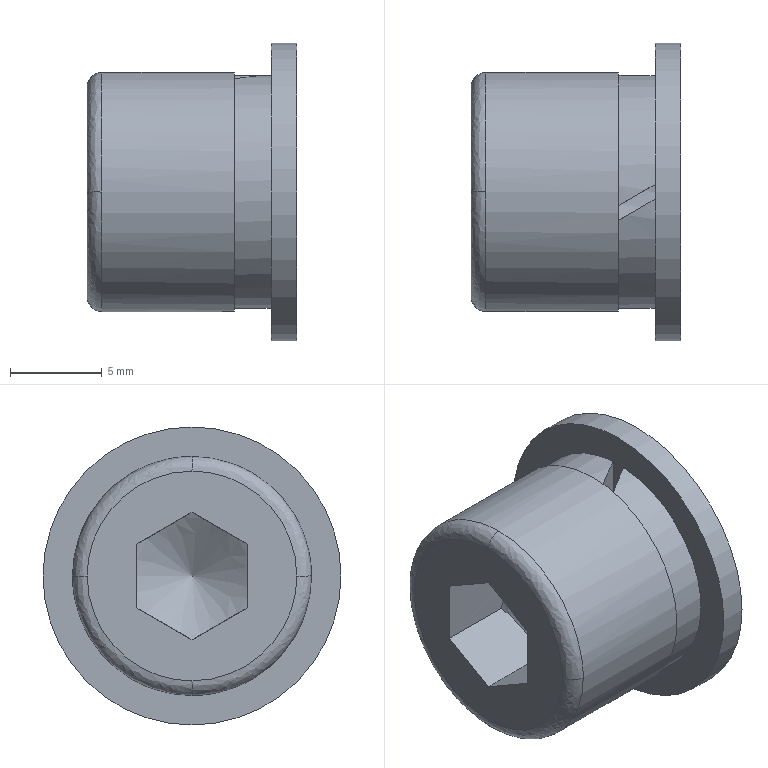Part | NX | features BREP 2 | 2 solids | 23 faces | box 11.4 x 16.2 x 16.2 mm | volume 1258 mm3 | plane 13 | cylinder 5 | spline 4 | cone 1 | commonest cylinder face diameters 8.2 x1 8.5 x1 12.7 x1 13 x1 16.2 x1
STEP:
#1=CARTESIAN_POINT('',(107.83,196.653,4.1));
#2=VERTEX_POINT('',#1);
#3=CARTESIAN_POINT('',(107.83,196.653,0.));
#4=DIRECTION('',(-1.,0.,0.));
#5=DIRECTION('',(0.,0.,1.));
#6=AXIS2_PLACEMENT_3D('',#3,#4,#5);
#7=CIRCLE('',#6,4.1);
#8=EDGE_CURVE('',#2,#2,#7,.T.);
#9=ORIENTED_EDGE('',*,*,#8,.T.);
#10=EDGE_LOOP('',(#9));
#11=FACE_BOUND('',#10,.T.);
#12=CARTESIAN_POINT('',(107.83,196.653,8.1));
#13=VERTEX_POINT('',#12);
#14=CARTESIAN_POINT('',(107.83,196.653,0.));
#15=DIRECTION('',(-1.,0.,0.));
#16=DIRECTION('',(0.,0.,1.));
#17=AXIS2_PLACEMENT_3D('',#14,#15,#16);
#18=CIRCLE('',#17,8.1);
#19=EDGE_CURVE('',#13,#13,#18,.T.);
#20=ORIENTED_EDGE('',*,*,#19,.F.);
#21=EDGE_LOOP('',(#20));
#22=FACE_BOUND('',#21,.T.);
#23=CARTESIAN_POINT('',(107.83,204.753,0.));
#24=DIRECTION('',(-1.,0.,0.));
#25=DIRECTION('',(0.,0.,-1.));
#26=AXIS2_PLACEMENT_3D('',#23,#24,#25);
#27=PLANE('',#26);
#28=ADVANCED_FACE('',(#11,#22),#27,.F.);
#29=CARTESIAN_POINT('',(106.43,196.653,4.1));
#30=VERTEX_POINT('',#29);
#31=CARTESIAN_POINT('',(106.43,196.653,0.));
#32=DIRECTION('',(-1.,0.,0.));
#33=DIRECTION('',(0.,0.,1.));
#34=AXIS2_PLACEMENT_3D('',#31,#32,#33);
#35=CIRCLE('',#34,4.1);
#36=EDGE_CURVE('',#30,#30,#35,.T.);
#37=ORIENTED_EDGE('',*,*,#36,.F.);
#38=EDGE_LOOP('',(#37));
#39=FACE_BOUND('',#38,.T.);
#40=CARTESIAN_POINT('',(106.43,196.653,8.1));
#41=VERTEX_POINT('',#40);
#42=CARTESIAN_POINT('',(106.43,196.653,0.));
#43=DIRECTION('',(-1.,0.,0.));
#44=DIRECTION('',(0.,0.,1.));
#45=AXIS2_PLACEMENT_3D('',#42,#43,#44);
#46=CIRCLE('',#45,8.1);
#47=EDGE_CURVE('',#41,#41,#46,.T.);
#48=ORIENTED_EDGE('',*,*,#47,.T.);
#49=EDGE_LOOP('',(#48));
#50=FACE_BOUND('',#49,.T.);
#51=CARTESIAN_POINT('',(106.43,200.753,0.));
#52=DIRECTION('',(-1.,0.,0.));
#53=DIRECTION('',(0.,0.,-1.));
#54=AXIS2_PLACEMENT_3D('',#51,#52,#53);
#55=PLANE('',#54);
#56=ADVANCED_FACE('',(#39,#50),#55,.T.);
#57=ORIENTED_EDGE('',*,*,#36,.T.);
#58=EDGE_LOOP('',(#57));
#59=FACE_BOUND('',#58,.T.);
#60=ORIENTED_EDGE('',*,*,#8,.F.);
#61=EDGE_LOOP('',(#60));
#62=FACE_BOUND('',#61,.T.);
#63=CARTESIAN_POINT('',(107.13,196.653,0.));
#64=DIRECTION('',(-1.,0.,0.));
#65=DIRECTION('',(0.,0.,-1.));
#66=AXIS2_PLACEMENT_3D('',#63,#64,#65);
#67=CYLINDRICAL_SURFACE('',#66,4.1);
#68=ADVANCED_FACE('',(#59,#62),#67,.F.);
#69=ORIENTED_EDGE('',*,*,#19,.T.);
#70=EDGE_LOOP('',(#69));
#71=FACE_BOUND('',#70,.T.);
#72=ORIENTED_EDGE('',*,*,#47,.F.);
#73=EDGE_LOOP('',(#72));
#74=FACE_BOUND('',#73,.T.);
#75=CARTESIAN_POINT('',(107.13,196.653,0.));
#76=DIRECTION('',(-1.,0.,0.));
#77=DIRECTION('',(0.,0.,-1.));
#78=AXIS2_PLACEMENT_3D('',#75,#76,#77);
#79=CYLINDRICAL_SURFACE('',#78,8.1);
#80=ADVANCED_FACE('',(#71,#74),#79,.T.);
#81=CLOSED_SHELL('',(#28,#56,#68,#80));
#82=MANIFOLD_SOLID_BREP('',#81);
#83=CARTESIAN_POINT('',(102.43,196.653,0.));
#84=VERTEX_POINT('',#83);
#85=VERTEX_LOOP('',#84);
#86=FACE_BOUND('',#85,.T.);
#87=CARTESIAN_POINT('',(100.43,193.653,-1.734));
#88=VERTEX_POINT('',#87);
#89=CARTESIAN_POINT('',(100.43,193.653,1.734));
#90=VERTEX_POINT('',#89);
#91=CARTESIAN_POINT('',(100.43,193.653,-1.734));
#92=CARTESIAN_POINT('',(100.757,193.653,-0.6009));
#93=CARTESIAN_POINT('',(100.757,193.653,0.6009));
#94=CARTESIAN_POINT('',(100.43,193.653,1.734));
#95=B_SPLINE_CURVE_WITH_KNOTS('',3,(#91,#92,#93,#94),.UNSPECIFIED.,.F.,.F.,(4,4),(0.,0.003509),.UNSPECIFIED.);
#96=EDGE_CURVE('',#88,#90,#95,.T.);
#97=ORIENTED_EDGE('',*,*,#96,.T.);
#98=CARTESIAN_POINT('',(100.43,196.653,3.465));
#99=VERTEX_POINT('',#98);
#100=CARTESIAN_POINT('',(100.43,193.653,1.734));
#101=CARTESIAN_POINT('',(100.756,194.632,2.299));
#102=CARTESIAN_POINT('',(100.756,195.672,2.899));
#103=CARTESIAN_POINT('',(100.43,196.653,3.465));
#104=B_SPLINE_CURVE_WITH_KNOTS('',3,(#100,#101,#102,#103),.UNSPECIFIED.,.F.,.F.,(4,4),(0.,0.003498),.UNSPECIFIED.);
#105=EDGE_CURVE('',#90,#99,#104,.T.);
#106=ORIENTED_EDGE('',*,*,#105,.T.);
#107=CARTESIAN_POINT('',(100.43,199.653,1.734));
#108=VERTEX_POINT('',#107);
#109=CARTESIAN_POINT('',(100.43,196.653,3.465));
#110=CARTESIAN_POINT('',(100.756,197.632,2.9));
#111=CARTESIAN_POINT('',(100.756,198.672,2.3));
#112=CARTESIAN_POINT('',(100.43,199.653,1.734));
#113=B_SPLINE_CURVE_WITH_KNOTS('',3,(#109,#110,#111,#112),.UNSPECIFIED.,.F.,.F.,(4,4),(0.,0.003498),.UNSPECIFIED.);
#114=EDGE_CURVE('',#99,#108,#113,.T.);
#115=ORIENTED_EDGE('',*,*,#114,.T.);
#116=CARTESIAN_POINT('',(100.43,199.653,-1.734));
#117=VERTEX_POINT('',#116);
#118=CARTESIAN_POINT('',(100.43,199.653,1.734));
#119=CARTESIAN_POINT('',(100.757,199.653,0.6009));
#120=CARTESIAN_POINT('',(100.757,199.653,-0.6009));
#121=CARTESIAN_POINT('',(100.43,199.653,-1.734));
#122=B_SPLINE_CURVE_WITH_KNOTS('',3,(#118,#119,#120,#121),.UNSPECIFIED.,.F.,.F.,(4,4),(0.,0.003509),.UNSPECIFIED.);
#123=EDGE_CURVE('',#108,#117,#122,.T.);
#124=ORIENTED_EDGE('',*,*,#123,.T.);
#125=CARTESIAN_POINT('',(100.43,196.653,-3.465));
#126=VERTEX_POINT('',#125);
#127=CARTESIAN_POINT('',(100.43,199.653,-1.734));
#128=CARTESIAN_POINT('',(100.756,198.673,-2.299));
#129=CARTESIAN_POINT('',(100.756,197.634,-2.899));
#130=CARTESIAN_POINT('',(100.43,196.653,-3.465));
#131=B_SPLINE_CURVE_WITH_KNOTS('',3,(#127,#128,#129,#130),.UNSPECIFIED.,.F.,.F.,(4,4),(0.,0.003498),.UNSPECIFIED.);
#132=EDGE_CURVE('',#117,#126,#131,.T.);
#133=ORIENTED_EDGE('',*,*,#132,.T.);
#134=CARTESIAN_POINT('',(100.43,196.653,-3.465));
#135=CARTESIAN_POINT('',(100.756,195.673,-2.9));
#136=CARTESIAN_POINT('',(100.756,194.634,-2.3));
#137=CARTESIAN_POINT('',(100.43,193.653,-1.734));
#138=B_SPLINE_CURVE_WITH_KNOTS('',3,(#134,#135,#136,#137),.UNSPECIFIED.,.F.,.F.,(4,4),(0.,0.003498),.UNSPECIFIED.);
#139=EDGE_CURVE('',#126,#88,#138,.T.);
#140=ORIENTED_EDGE('',*,*,#139,.T.);
#141=EDGE_LOOP('',(#97,#106,#115,#124,#133,#140));
#142=FACE_BOUND('',#141,.T.);
#143=CARTESIAN_POINT('',(101.43,196.653,0.));
#144=DIRECTION('',(-1.,0.,0.));
#145=DIRECTION('',(0.,1.,0.));
#146=AXIS2_PLACEMENT_3D('',#143,#144,#145);
#147=CONICAL_SURFACE('',#146,1.733,1.047);
#148=ADVANCED_FACE('',(#86,#142),#147,.F.);
#149=ORIENTED_EDGE('',*,*,#123,.F.);
#150=CARTESIAN_POINT('',(96.43,199.653,1.734));
#151=VERTEX_POINT('',#150);
#152=CARTESIAN_POINT('',(96.43,199.653,1.734));
#153=DIRECTION('',(1.,0.,0.));
#154=VECTOR('',#153,1000.);
#155=LINE('',#152,#154);
#156=EDGE_CURVE('',#151,#108,#155,.T.);
#157=ORIENTED_EDGE('',*,*,#156,.F.);
#158=CARTESIAN_POINT('',(96.43,199.653,-1.734));
#159=VERTEX_POINT('',#158);
#160=CARTESIAN_POINT('',(96.43,199.653,0.));
#161=DIRECTION('',(0.,0.,1.));
#162=VECTOR('',#161,1000.);
#163=LINE('',#160,#162);
#164=EDGE_CURVE('',#159,#151,#163,.T.);
#165=ORIENTED_EDGE('',*,*,#164,.F.);
#166=CARTESIAN_POINT('',(96.43,199.653,-1.734));
#167=DIRECTION('',(1.,0.,0.));
#168=VECTOR('',#167,1000.);
#169=LINE('',#166,#168);
#170=EDGE_CURVE('',#159,#117,#169,.T.);
#171=ORIENTED_EDGE('',*,*,#170,.T.);
#172=EDGE_LOOP('',(#149,#157,#165,#171));
#173=FACE_BOUND('',#172,.T.);
#174=CARTESIAN_POINT('',(96.43,199.653,-1.734));
#175=DIRECTION('',(0.,-1.,0.));
#176=DIRECTION('',(0.,0.,-1.));
#177=AXIS2_PLACEMENT_3D('',#174,#175,#176);
#178=PLANE('',#177);
#179=ADVANCED_FACE('',(#173),#178,.T.);
#180=ORIENTED_EDGE('',*,*,#132,.F.);
#181=ORIENTED_EDGE('',*,*,#170,.F.);
#182=CARTESIAN_POINT('',(96.43,196.653,-3.465));
#183=VERTEX_POINT('',#182);
#184=CARTESIAN_POINT('',(96.43,201.891,-0.4425));
#185=DIRECTION('',(0.,0.8661,0.4998));
#186=VECTOR('',#185,1000.);
#187=LINE('',#184,#186);
#188=EDGE_CURVE('',#183,#159,#187,.T.);
#189=ORIENTED_EDGE('',*,*,#188,.F.);
#190=CARTESIAN_POINT('',(96.43,196.653,-3.465));
#191=DIRECTION('',(-1.,0.,0.));
#192=VECTOR('',#191,1000.);
#193=LINE('',#190,#192);
#194=EDGE_CURVE('',#126,#183,#193,.T.);
#195=ORIENTED_EDGE('',*,*,#194,.F.);
#196=EDGE_LOOP('',(#180,#181,#189,#195));
#197=FACE_BOUND('',#196,.T.);
#198=CARTESIAN_POINT('',(96.43,196.653,-3.465));
#199=DIRECTION('',(0.,-0.4998,0.8661));
#200=DIRECTION('',(1.,0.,0.));
#201=AXIS2_PLACEMENT_3D('',#198,#199,#200);
#202=PLANE('',#201);
#203=ADVANCED_FACE('',(#197),#202,.T.);
#204=ORIENTED_EDGE('',*,*,#139,.F.);
#205=ORIENTED_EDGE('',*,*,#194,.T.);
#206=CARTESIAN_POINT('',(96.43,193.653,-1.734));
#207=VERTEX_POINT('',#206);
#208=CARTESIAN_POINT('',(96.43,198.891,-4.756));
#209=DIRECTION('',(0.,0.8661,-0.4998));
#210=VECTOR('',#209,1000.);
#211=LINE('',#208,#210);
#212=EDGE_CURVE('',#207,#183,#211,.T.);
#213=ORIENTED_EDGE('',*,*,#212,.F.);
#214=CARTESIAN_POINT('',(96.43,193.653,-1.734));
#215=DIRECTION('',(1.,0.,0.));
#216=VECTOR('',#215,1000.);
#217=LINE('',#214,#216);
#218=EDGE_CURVE('',#207,#88,#217,.T.);
#219=ORIENTED_EDGE('',*,*,#218,.T.);
#220=EDGE_LOOP('',(#204,#205,#213,#219));
#221=FACE_BOUND('',#220,.T.);
#222=CARTESIAN_POINT('',(96.43,193.653,-1.734));
#223=DIRECTION('',(0.,0.4998,0.8661));
#224=DIRECTION('',(1.,0.,0.));
#225=AXIS2_PLACEMENT_3D('',#222,#223,#224);
#226=PLANE('',#225);
#227=ADVANCED_FACE('',(#221),#226,.T.);
#228=ORIENTED_EDGE('',*,*,#96,.F.);
#229=ORIENTED_EDGE('',*,*,#218,.F.);
#230=CARTESIAN_POINT('',(96.43,193.653,1.734));
#231=VERTEX_POINT('',#230);
#232=CARTESIAN_POINT('',(96.43,193.653,0.));
#233=DIRECTION('',(0.,0.,-1.));
#234=VECTOR('',#233,1000.);
#235=LINE('',#232,#234);
#236=EDGE_CURVE('',#231,#207,#235,.T.);
#237=ORIENTED_EDGE('',*,*,#236,.F.);
#238=CARTESIAN_POINT('',(96.43,193.653,1.734));
#239=DIRECTION('',(1.,0.,0.));
#240=VECTOR('',#239,1000.);
#241=LINE('',#238,#240);
#242=EDGE_CURVE('',#231,#90,#241,.T.);
#243=ORIENTED_EDGE('',*,*,#242,.T.);
#244=EDGE_LOOP('',(#228,#229,#237,#243));
#245=FACE_BOUND('',#244,.T.);
#246=CARTESIAN_POINT('',(96.43,193.653,1.734));
#247=DIRECTION('',(0.,1.,0.));
#248=DIRECTION('',(0.,0.,1.));
#249=AXIS2_PLACEMENT_3D('',#246,#247,#248);
#250=PLANE('',#249);
#251=ADVANCED_FACE('',(#245),#250,.T.);
#252=ORIENTED_EDGE('',*,*,#105,.F.);
#253=ORIENTED_EDGE('',*,*,#242,.F.);
#254=CARTESIAN_POINT('',(96.43,196.653,3.465));
#255=VERTEX_POINT('',#254);
#256=CARTESIAN_POINT('',(96.43,198.891,4.756));
#257=DIRECTION('',(0.,-0.8661,-0.4998));
#258=VECTOR('',#257,1000.);
#259=LINE('',#256,#258);
#260=EDGE_CURVE('',#255,#231,#259,.T.);
#261=ORIENTED_EDGE('',*,*,#260,.F.);
#262=CARTESIAN_POINT('',(96.43,196.653,3.465));
#263=DIRECTION('',(1.,0.,0.));
#264=VECTOR('',#263,1000.);
#265=LINE('',#262,#264);
#266=EDGE_CURVE('',#255,#99,#265,.T.);
#267=ORIENTED_EDGE('',*,*,#266,.T.);
#268=EDGE_LOOP('',(#252,#253,#261,#267));
#269=FACE_BOUND('',#268,.T.);
#270=CARTESIAN_POINT('',(96.43,196.653,3.465));
#271=DIRECTION('',(0.,0.4998,-0.8661));
#272=DIRECTION('',(-1.,0.,0.));
#273=AXIS2_PLACEMENT_3D('',#270,#271,#272);
#274=PLANE('',#273);
#275=ADVANCED_FACE('',(#269),#274,.T.);
#276=ORIENTED_EDGE('',*,*,#114,.F.);
#277=ORIENTED_EDGE('',*,*,#266,.F.);
#278=CARTESIAN_POINT('',(96.43,201.891,0.4425));
#279=DIRECTION('',(0.,-0.8661,0.4998));
#280=VECTOR('',#279,1000.);
#281=LINE('',#278,#280);
#282=EDGE_CURVE('',#151,#255,#281,.T.);
#283=ORIENTED_EDGE('',*,*,#282,.F.);
#284=ORIENTED_EDGE('',*,*,#156,.T.);
#285=EDGE_LOOP('',(#276,#277,#283,#284));
#286=FACE_BOUND('',#285,.T.);
#287=CARTESIAN_POINT('',(96.43,199.653,1.734));
#288=DIRECTION('',(0.,-0.4998,-0.8661));
#289=DIRECTION('',(-1.,0.,0.));
#290=AXIS2_PLACEMENT_3D('',#287,#288,#289);
#291=PLANE('',#290);
#292=ADVANCED_FACE('',(#286),#291,.T.);
#293=ORIENTED_EDGE('',*,*,#282,.T.);
#294=ORIENTED_EDGE('',*,*,#260,.T.);
#295=ORIENTED_EDGE('',*,*,#236,.T.);
#296=ORIENTED_EDGE('',*,*,#212,.T.);
#297=ORIENTED_EDGE('',*,*,#188,.T.);
#298=ORIENTED_EDGE('',*,*,#164,.T.);
#299=EDGE_LOOP('',(#293,#294,#295,#296,#297,#298));
#300=FACE_BOUND('',#299,.T.);
#301=CARTESIAN_POINT('',(96.43,202.353,0.));
#302=VERTEX_POINT('',#301);
#303=CARTESIAN_POINT('',(96.43,196.653,-5.7));
#304=VERTEX_POINT('',#303);
#305=CARTESIAN_POINT('',(96.43,202.353,0.));
#306=CARTESIAN_POINT('',(96.43,202.353,-1.492));
#307=CARTESIAN_POINT('',(96.43,201.118,-4.465));
#308=CARTESIAN_POINT('',(96.43,198.145,-5.7));
#309=CARTESIAN_POINT('',(96.43,196.653,-5.7));
#310=B_SPLINE_CURVE_WITH_KNOTS('',3,(#305,#306,#307,#308,#309),.UNSPECIFIED.,.F.,.F.,(4,1,4),(0.,6.331,12.662),.UNSPECIFIED.);
#311=EDGE_CURVE('',#302,#304,#310,.T.);
#312=ORIENTED_EDGE('',*,*,#311,.T.);
#313=CARTESIAN_POINT('',(96.43,190.953,0.));
#314=VERTEX_POINT('',#313);
#315=CARTESIAN_POINT('',(96.43,196.653,-5.7));
#316=CARTESIAN_POINT('',(96.43,195.16,-5.7));
#317=CARTESIAN_POINT('',(96.43,192.188,-4.465));
#318=CARTESIAN_POINT('',(96.43,190.953,-1.492));
#319=CARTESIAN_POINT('',(96.43,190.953,0.));
#320=B_SPLINE_CURVE_WITH_KNOTS('',3,(#315,#316,#317,#318,#319),.UNSPECIFIED.,.F.,.F.,(4,1,4),(0.,6.331,12.662),.UNSPECIFIED.);
#321=EDGE_CURVE('',#304,#314,#320,.T.);
#322=ORIENTED_EDGE('',*,*,#321,.T.);
#323=CARTESIAN_POINT('',(96.43,196.653,5.7));
#324=VERTEX_POINT('',#323);
#325=CARTESIAN_POINT('',(96.43,190.953,0.));
#326=CARTESIAN_POINT('',(96.43,190.953,1.492));
#327=CARTESIAN_POINT('',(96.43,192.188,4.465));
#328=CARTESIAN_POINT('',(96.43,195.16,5.7));
#329=CARTESIAN_POINT('',(96.43,196.653,5.7));
#330=B_SPLINE_CURVE_WITH_KNOTS('',3,(#325,#326,#327,#328,#329),.UNSPECIFIED.,.F.,.F.,(4,1,4),(12.662,18.993,25.324),.UNSPECIFIED.);
#331=EDGE_CURVE('',#314,#324,#330,.T.);
#332=ORIENTED_EDGE('',*,*,#331,.T.);
#333=CARTESIAN_POINT('',(96.43,196.653,5.7));
#334=CARTESIAN_POINT('',(96.43,198.145,5.7));
#335=CARTESIAN_POINT('',(96.43,201.118,4.465));
#336=CARTESIAN_POINT('',(96.43,202.353,1.492));
#337=CARTESIAN_POINT('',(96.43,202.353,0.));
#338=B_SPLINE_CURVE_WITH_KNOTS('',3,(#333,#334,#335,#336,#337),.UNSPECIFIED.,.F.,.F.,(4,1,4),(0.,6.331,12.662),.UNSPECIFIED.);
#339=EDGE_CURVE('',#324,#302,#338,.T.);
#340=ORIENTED_EDGE('',*,*,#339,.T.);
#341=EDGE_LOOP('',(#312,#322,#332,#340));
#342=FACE_BOUND('',#341,.T.);
#343=CARTESIAN_POINT('',(96.43,201.635,0.));
#344=DIRECTION('',(-1.,0.,0.));
#345=DIRECTION('',(0.,0.,1.));
#346=AXIS2_PLACEMENT_3D('',#343,#344,#345);
#347=PLANE('',#346);
#348=ADVANCED_FACE('',(#300,#342),#347,.T.);
#349=CARTESIAN_POINT('',(97.23,203.153,0.));
#350=VERTEX_POINT('',#349);
#351=CARTESIAN_POINT('',(97.23,196.653,-6.5));
#352=VERTEX_POINT('',#351);
#353=CARTESIAN_POINT('',(97.23,196.653,-6.5));
#354=CARTESIAN_POINT('',(97.23,198.354,-6.5));
#355=CARTESIAN_POINT('',(97.23,201.744,-5.092));
#356=CARTESIAN_POINT('',(97.23,203.153,-1.702));
#357=CARTESIAN_POINT('',(97.23,203.153,0.));
#358=B_SPLINE_CURVE_WITH_KNOTS('',3,(#353,#354,#355,#356,#357),.UNSPECIFIED.,.F.,.F.,(4,1,4),(0.,5.105,10.21),.UNSPECIFIED.);
#359=EDGE_CURVE('',#350,#352,#358,.F.);
#360=ORIENTED_EDGE('',*,*,#359,.T.);
#361=CARTESIAN_POINT('',(97.23,196.653,-6.5));
#362=CARTESIAN_POINT('',(97.041,196.653,-6.5));
#363=CARTESIAN_POINT('',(96.593,196.653,-6.337));
#364=CARTESIAN_POINT('',(96.43,196.653,-5.889));
#365=CARTESIAN_POINT('',(96.43,196.653,-5.7));
#366=B_SPLINE_CURVE_WITH_KNOTS('',3,(#361,#362,#363,#364,#365),.UNSPECIFIED.,.F.,.F.,(4,1,4),(0.,0.8736,1.747),.UNSPECIFIED.);
#367=EDGE_CURVE('',#352,#304,#366,.T.);
#368=ORIENTED_EDGE('',*,*,#367,.T.);
#369=ORIENTED_EDGE('',*,*,#311,.F.);
#370=CARTESIAN_POINT('',(96.43,202.353,0.));
#371=CARTESIAN_POINT('',(96.43,202.541,0.));
#372=CARTESIAN_POINT('',(96.593,202.99,0.));
#373=CARTESIAN_POINT('',(97.041,203.153,0.));
#374=CARTESIAN_POINT('',(97.23,203.153,0.));
#375=B_SPLINE_CURVE_WITH_KNOTS('',3,(#370,#371,#372,#373,#374),.UNSPECIFIED.,.F.,.F.,(4,1,4),(0.,0.8736,1.747),.UNSPECIFIED.);
#376=EDGE_CURVE('',#302,#350,#375,.T.);
#377=ORIENTED_EDGE('',*,*,#376,.T.);
#378=EDGE_LOOP('',(#360,#368,#369,#377));
#379=FACE_BOUND('',#378,.T.);
#380=CARTESIAN_POINT('',(97.23,203.153,0.));
#381=CARTESIAN_POINT('',(97.23,203.153,-6.5));
#382=CARTESIAN_POINT('',(97.23,196.653,-6.5));
#383=CARTESIAN_POINT('',(96.43,203.153,0.));
#384=CARTESIAN_POINT('',(96.43,203.153,-6.5));
#385=CARTESIAN_POINT('',(96.43,196.653,-6.5));
#386=CARTESIAN_POINT('',(96.43,202.353,0.));
#387=CARTESIAN_POINT('',(96.43,202.353,-5.7));
#388=CARTESIAN_POINT('',(96.43,196.653,-5.7));
#389=(BOUNDED_SURFACE()B_SPLINE_SURFACE(2,2,((#380,#381,#382),(#383,#384,#385),(#386,#387,#388)),.TOROIDAL_SURF.,.F.,.F.,.F.)B_SPLINE_SURFACE_WITH_KNOTS((3,3),(3,3),(0.,1.747),(34.2,45.6),.PIECEWISE_BEZIER_KNOTS.)GEOMETRIC_REPRESENTATION_ITEM()RATIONAL_B_SPLINE_SURFACE(((1.,0.7071,1.),(0.7071,0.5,0.7071),(1.,0.7071,1.)))REPRESENTATION_ITEM('')SURFACE());
#390=ADVANCED_FACE('',(#379),#389,.F.);
#391=ORIENTED_EDGE('',*,*,#321,.F.);
#392=ORIENTED_EDGE('',*,*,#367,.F.);
#393=CARTESIAN_POINT('',(97.23,190.153,0.));
#394=VERTEX_POINT('',#393);
#395=CARTESIAN_POINT('',(97.23,190.153,0.));
#396=CARTESIAN_POINT('',(97.23,190.153,-1.702));
#397=CARTESIAN_POINT('',(97.23,191.561,-5.092));
#398=CARTESIAN_POINT('',(97.23,194.951,-6.5));
#399=CARTESIAN_POINT('',(97.23,196.653,-6.5));
#400=B_SPLINE_CURVE_WITH_KNOTS('',3,(#395,#396,#397,#398,#399),.UNSPECIFIED.,.F.,.F.,(4,1,4),(10.21,15.315,20.42),.UNSPECIFIED.);
#401=EDGE_CURVE('',#352,#394,#400,.F.);
#402=ORIENTED_EDGE('',*,*,#401,.T.);
#403=CARTESIAN_POINT('',(97.23,190.153,0.));
#404=CARTESIAN_POINT('',(97.041,190.153,0.));
#405=CARTESIAN_POINT('',(96.593,190.316,0.));
#406=CARTESIAN_POINT('',(96.43,190.764,0.));
#407=CARTESIAN_POINT('',(96.43,190.953,0.));
#408=B_SPLINE_CURVE_WITH_KNOTS('',3,(#403,#404,#405,#406,#407),.UNSPECIFIED.,.F.,.F.,(4,1,4),(-0.8736,0.,0.8736),.UNSPECIFIED.);
#409=EDGE_CURVE('',#314,#394,#408,.F.);
#410=ORIENTED_EDGE('',*,*,#409,.F.);
#411=EDGE_LOOP('',(#391,#392,#402,#410));
#412=FACE_BOUND('',#411,.T.);
#413=CARTESIAN_POINT('',(97.23,196.653,-6.5));
#414=CARTESIAN_POINT('',(97.23,190.153,-6.5));
#415=CARTESIAN_POINT('',(97.23,190.153,0.));
#416=CARTESIAN_POINT('',(96.43,196.653,-6.5));
#417=CARTESIAN_POINT('',(96.43,190.153,-6.5));
#418=CARTESIAN_POINT('',(96.43,190.153,0.));
#419=CARTESIAN_POINT('',(96.43,196.653,-5.7));
#420=CARTESIAN_POINT('',(96.43,190.953,-5.7));
#421=CARTESIAN_POINT('',(96.43,190.953,0.));
#422=(BOUNDED_SURFACE()B_SPLINE_SURFACE(2,2,((#413,#414,#415),(#416,#417,#418),(#419,#420,#421)),.TOROIDAL_SURF.,.F.,.F.,.F.)B_SPLINE_SURFACE_WITH_KNOTS((3,3),(3,3),(0.,1.747),(0.,11.4),.PIECEWISE_BEZIER_KNOTS.)GEOMETRIC_REPRESENTATION_ITEM()RATIONAL_B_SPLINE_SURFACE(((1.,0.7071,1.),(0.7071,0.5,0.7071),(1.,0.7071,1.)))REPRESENTATION_ITEM('')SURFACE());
#423=ADVANCED_FACE('',(#412),#422,.F.);
#424=CARTESIAN_POINT('',(97.23,196.653,6.5));
#425=VERTEX_POINT('',#424);
#426=CARTESIAN_POINT('',(97.23,196.653,6.5));
#427=CARTESIAN_POINT('',(97.23,194.951,6.5));
#428=CARTESIAN_POINT('',(97.23,191.561,5.092));
#429=CARTESIAN_POINT('',(97.23,190.153,1.702));
#430=CARTESIAN_POINT('',(97.23,190.153,0.));
#431=B_SPLINE_CURVE_WITH_KNOTS('',3,(#426,#427,#428,#429,#430),.UNSPECIFIED.,.F.,.F.,(4,1,4),(-5.105,0.,5.105),.UNSPECIFIED.);
#432=EDGE_CURVE('',#394,#425,#431,.F.);
#433=ORIENTED_EDGE('',*,*,#432,.T.);
#434=CARTESIAN_POINT('',(97.23,196.653,6.5));
#435=CARTESIAN_POINT('',(97.041,196.653,6.5));
#436=CARTESIAN_POINT('',(96.593,196.653,6.337));
#437=CARTESIAN_POINT('',(96.43,196.653,5.889));
#438=CARTESIAN_POINT('',(96.43,196.653,5.7));
#439=B_SPLINE_CURVE_WITH_KNOTS('',3,(#434,#435,#436,#437,#438),.UNSPECIFIED.,.F.,.F.,(4,1,4),(-0.8736,0.,0.8736),.UNSPECIFIED.);
#440=EDGE_CURVE('',#324,#425,#439,.F.);
#441=ORIENTED_EDGE('',*,*,#440,.F.);
#442=ORIENTED_EDGE('',*,*,#331,.F.);
#443=ORIENTED_EDGE('',*,*,#409,.T.);
#444=EDGE_LOOP('',(#433,#441,#442,#443));
#445=FACE_BOUND('',#444,.T.);
#446=CARTESIAN_POINT('',(97.23,190.153,0.));
#447=CARTESIAN_POINT('',(97.23,190.153,6.5));
#448=CARTESIAN_POINT('',(97.23,196.653,6.5));
#449=CARTESIAN_POINT('',(96.43,190.153,0.));
#450=CARTESIAN_POINT('',(96.43,190.153,6.5));
#451=CARTESIAN_POINT('',(96.43,196.653,6.5));
#452=CARTESIAN_POINT('',(96.43,190.953,0.));
#453=CARTESIAN_POINT('',(96.43,190.953,5.7));
#454=CARTESIAN_POINT('',(96.43,196.653,5.7));
#455=(BOUNDED_SURFACE()B_SPLINE_SURFACE(2,2,((#446,#447,#448),(#449,#450,#451),(#452,#453,#454)),.TOROIDAL_SURF.,.F.,.F.,.F.)B_SPLINE_SURFACE_WITH_KNOTS((3,3),(3,3),(0.,1.747),(11.4,22.8),.PIECEWISE_BEZIER_KNOTS.)GEOMETRIC_REPRESENTATION_ITEM()RATIONAL_B_SPLINE_SURFACE(((1.,0.7071,1.),(0.7071,0.5,0.7071),(1.,0.7071,1.)))REPRESENTATION_ITEM('')SURFACE());
#456=ADVANCED_FACE('',(#445),#455,.F.);
#457=ORIENTED_EDGE('',*,*,#339,.F.);
#458=ORIENTED_EDGE('',*,*,#440,.T.);
#459=CARTESIAN_POINT('',(97.23,203.153,0.));
#460=CARTESIAN_POINT('',(97.23,203.153,1.702));
#461=CARTESIAN_POINT('',(97.23,201.744,5.092));
#462=CARTESIAN_POINT('',(97.23,198.354,6.5));
#463=CARTESIAN_POINT('',(97.23,196.653,6.5));
#464=B_SPLINE_CURVE_WITH_KNOTS('',3,(#459,#460,#461,#462,#463),.UNSPECIFIED.,.F.,.F.,(4,1,4),(30.631,35.736,40.841),.UNSPECIFIED.);
#465=EDGE_CURVE('',#425,#350,#464,.F.);
#466=ORIENTED_EDGE('',*,*,#465,.T.);
#467=ORIENTED_EDGE('',*,*,#376,.F.);
#468=EDGE_LOOP('',(#457,#458,#466,#467));
#469=FACE_BOUND('',#468,.T.);
#470=CARTESIAN_POINT('',(97.23,196.653,6.5));
#471=CARTESIAN_POINT('',(97.23,203.153,6.5));
#472=CARTESIAN_POINT('',(97.23,203.153,0.));
#473=CARTESIAN_POINT('',(96.43,196.653,6.5));
#474=CARTESIAN_POINT('',(96.43,203.153,6.5));
#475=CARTESIAN_POINT('',(96.43,203.153,0.));
#476=CARTESIAN_POINT('',(96.43,196.653,5.7));
#477=CARTESIAN_POINT('',(96.43,202.353,5.7));
#478=CARTESIAN_POINT('',(96.43,202.353,0.));
#479=(BOUNDED_SURFACE()B_SPLINE_SURFACE(2,2,((#470,#471,#472),(#473,#474,#475),(#476,#477,#478)),.TOROIDAL_SURF.,.F.,.F.,.F.)B_SPLINE_SURFACE_WITH_KNOTS((3,3),(3,3),(0.,1.747),(22.8,34.2),.PIECEWISE_BEZIER_KNOTS.)GEOMETRIC_REPRESENTATION_ITEM()RATIONAL_B_SPLINE_SURFACE(((1.,0.7071,1.),(0.7071,0.5,0.7071),(1.,0.7071,1.)))REPRESENTATION_ITEM('')SURFACE());
#480=ADVANCED_FACE('',(#469),#479,.F.);
#481=ORIENTED_EDGE('',*,*,#359,.F.);
#482=ORIENTED_EDGE('',*,*,#465,.F.);
#483=ORIENTED_EDGE('',*,*,#432,.F.);
#484=ORIENTED_EDGE('',*,*,#401,.F.);
#485=EDGE_LOOP('',(#481,#482,#483,#484));
#486=FACE_BOUND('',#485,.T.);
#487=CARTESIAN_POINT('',(104.43,196.653,-6.5));
#488=VERTEX_POINT('',#487);
#489=CARTESIAN_POINT('',(104.43,196.653,0.));
#490=DIRECTION('',(1.,0.,0.));
#491=DIRECTION('',(0.,0.,-1.));
#492=AXIS2_PLACEMENT_3D('',#489,#490,#491);
#493=CIRCLE('',#492,6.5);
#494=EDGE_CURVE('',#488,#488,#493,.F.);
#495=ORIENTED_EDGE('',*,*,#494,.T.);
#496=EDGE_LOOP('',(#495));
#497=FACE_BOUND('',#496,.T.);
#498=CARTESIAN_POINT('',(100.43,196.653,0.));
#499=DIRECTION('',(-1.,0.,0.));
#500=DIRECTION('',(0.,1.,0.));
#501=AXIS2_PLACEMENT_3D('',#498,#499,#500);
#502=CYLINDRICAL_SURFACE('',#501,6.5);
#503=ADVANCED_FACE('',(#486,#497),#502,.T.);
#504=CARTESIAN_POINT('',(104.43,195.098,3.955));
#505=VERTEX_POINT('',#504);
#506=CARTESIAN_POINT('',(104.43,195.898,4.182));
#507=VERTEX_POINT('',#506);
#508=CARTESIAN_POINT('',(104.43,196.653,0.));
#509=DIRECTION('',(1.,0.,0.));
#510=DIRECTION('',(0.,0.,-1.));
#511=AXIS2_PLACEMENT_3D('',#508,#509,#510);
#512=CIRCLE('',#511,4.25);
#513=EDGE_CURVE('',#505,#507,#512,.T.);
#514=ORIENTED_EDGE('',*,*,#513,.T.);
#515=CARTESIAN_POINT('',(104.43,195.898,6.305));
#516=VERTEX_POINT('',#515);
#517=CARTESIAN_POINT('',(104.43,195.898,0.));
#518=DIRECTION('',(0.,0.,1.));
#519=VECTOR('',#518,1000.);
#520=LINE('',#517,#519);
#521=EDGE_CURVE('',#507,#516,#520,.T.);
#522=ORIENTED_EDGE('',*,*,#521,.T.);
#523=CARTESIAN_POINT('',(104.43,195.098,6.157));
#524=VERTEX_POINT('',#523);
#525=CARTESIAN_POINT('',(104.43,196.653,0.));
#526=DIRECTION('',(1.,0.,0.));
#527=DIRECTION('',(0.,0.,-1.));
#528=AXIS2_PLACEMENT_3D('',#525,#526,#527);
#529=CIRCLE('',#528,6.35);
#530=EDGE_CURVE('',#524,#516,#529,.T.);
#531=ORIENTED_EDGE('',*,*,#530,.F.);
#532=CARTESIAN_POINT('',(104.43,195.098,0.));
#533=DIRECTION('',(0.,0.,-1.));
#534=VECTOR('',#533,1000.);
#535=LINE('',#532,#534);
#536=EDGE_CURVE('',#524,#505,#535,.T.);
#537=ORIENTED_EDGE('',*,*,#536,.T.);
#538=EDGE_LOOP('',(#514,#522,#531,#537));
#539=FACE_BOUND('',#538,.T.);
#540=ORIENTED_EDGE('',*,*,#494,.F.);
#541=EDGE_LOOP('',(#540));
#542=FACE_BOUND('',#541,.T.);
#543=CARTESIAN_POINT('',(104.43,0.,0.));
#544=DIRECTION('',(1.,0.,0.));
#545=DIRECTION('',(0.,1.,0.));
#546=AXIS2_PLACEMENT_3D('',#543,#544,#545);
#547=PLANE('',#546);
#548=ADVANCED_FACE('',(#539,#542),#547,.T.);
#549=ORIENTED_EDGE('',*,*,#513,.F.);
#550=CARTESIAN_POINT('',(106.43,196.253,4.231));
#551=VERTEX_POINT('',#550);
#552=CARTESIAN_POINT('',(107.122,196.653,0.));
#553=DIRECTION('',(0.5,-0.866,0.));
#554=DIRECTION('',(0.866,0.5,0.));
#555=AXIS2_PLACEMENT_3D('',#552,#553,#554);
#556=ELLIPSE('',#555,8.5,4.25);
#557=EDGE_CURVE('',#505,#551,#556,.F.);
#558=ORIENTED_EDGE('',*,*,#557,.T.);
#559=CARTESIAN_POINT('',(106.43,197.053,4.231));
#560=VERTEX_POINT('',#559);
#561=CARTESIAN_POINT('',(106.43,196.653,0.));
#562=DIRECTION('',(1.,0.,0.));
#563=DIRECTION('',(0.,0.,-1.));
#564=AXIS2_PLACEMENT_3D('',#561,#562,#563);
#565=CIRCLE('',#564,4.25);
#566=EDGE_CURVE('',#551,#560,#565,.T.);
#567=ORIENTED_EDGE('',*,*,#566,.T.);
#568=CARTESIAN_POINT('',(105.737,196.653,0.));
#569=DIRECTION('',(-0.5,0.866,0.));
#570=DIRECTION('',(0.866,0.5,0.));
#571=AXIS2_PLACEMENT_3D('',#568,#569,#570);
#572=ELLIPSE('',#571,8.5,4.25);
#573=EDGE_CURVE('',#560,#507,#572,.F.);
#574=ORIENTED_EDGE('',*,*,#573,.T.);
#575=EDGE_LOOP('',(#549,#558,#567,#574));
#576=FACE_BOUND('',#575,.T.);
#577=CARTESIAN_POINT('',(105.43,196.653,0.));
#578=DIRECTION('',(1.,0.,0.));
#579=DIRECTION('',(0.,1.,0.));
#580=AXIS2_PLACEMENT_3D('',#577,#578,#579);
#581=CYLINDRICAL_SURFACE('',#580,4.25);
#582=ADVANCED_FACE('',(#576),#581,.F.);
#583=CARTESIAN_POINT('',(106.43,197.053,6.337));
#584=VERTEX_POINT('',#583);
#585=CARTESIAN_POINT('',(105.737,196.653,0.));
#586=DIRECTION('',(-0.5,0.866,0.));
#587=DIRECTION('',(0.866,0.5,0.));
#588=AXIS2_PLACEMENT_3D('',#585,#586,#587);
#589=ELLIPSE('',#588,12.7,6.35);
#590=EDGE_CURVE('',#516,#584,#589,.T.);
#591=ORIENTED_EDGE('',*,*,#590,.F.);
#592=ORIENTED_EDGE('',*,*,#521,.F.);
#593=ORIENTED_EDGE('',*,*,#573,.F.);
#594=CARTESIAN_POINT('',(106.43,197.053,0.));
#595=DIRECTION('',(0.,0.,-1.));
#596=VECTOR('',#595,1000.);
#597=LINE('',#594,#596);
#598=EDGE_CURVE('',#584,#560,#597,.T.);
#599=ORIENTED_EDGE('',*,*,#598,.F.);
#600=EDGE_LOOP('',(#591,#592,#593,#599));
#601=FACE_BOUND('',#600,.T.);
#602=CARTESIAN_POINT('',(104.43,195.898,0.));
#603=DIRECTION('',(-0.5,0.866,0.));
#604=DIRECTION('',(0.,0.,1.));
#605=AXIS2_PLACEMENT_3D('',#602,#603,#604);
#606=PLANE('',#605);
#607=ADVANCED_FACE('',(#601),#606,.F.);
#608=CARTESIAN_POINT('',(106.43,196.253,6.337));
#609=VERTEX_POINT('',#608);
#610=CARTESIAN_POINT('',(107.122,196.653,0.));
#611=DIRECTION('',(0.5,-0.866,0.));
#612=DIRECTION('',(0.866,0.5,0.));
#613=AXIS2_PLACEMENT_3D('',#610,#611,#612);
#614=ELLIPSE('',#613,12.7,6.35);
#615=EDGE_CURVE('',#609,#524,#614,.T.);
#616=ORIENTED_EDGE('',*,*,#615,.F.);
#617=CARTESIAN_POINT('',(106.43,196.253,0.));
#618=DIRECTION('',(0.,0.,1.));
#619=VECTOR('',#618,1000.);
#620=LINE('',#617,#619);
#621=EDGE_CURVE('',#551,#609,#620,.T.);
#622=ORIENTED_EDGE('',*,*,#621,.F.);
#623=ORIENTED_EDGE('',*,*,#557,.F.);
#624=ORIENTED_EDGE('',*,*,#536,.F.);
#625=EDGE_LOOP('',(#616,#622,#623,#624));
#626=FACE_BOUND('',#625,.T.);
#627=CARTESIAN_POINT('',(106.43,196.253,0.));
#628=DIRECTION('',(0.5,-0.866,0.));
#629=DIRECTION('',(0.,0.,-1.));
#630=AXIS2_PLACEMENT_3D('',#627,#628,#629);
#631=PLANE('',#630);
#632=ADVANCED_FACE('',(#626),#631,.F.);
#633=ORIENTED_EDGE('',*,*,#598,.T.);
#634=ORIENTED_EDGE('',*,*,#566,.F.);
#635=ORIENTED_EDGE('',*,*,#621,.T.);
#636=CARTESIAN_POINT('',(106.43,196.653,0.));
#637=DIRECTION('',(1.,0.,0.));
#638=DIRECTION('',(0.,0.,-1.));
#639=AXIS2_PLACEMENT_3D('',#636,#637,#638);
#640=CIRCLE('',#639,6.35);
#641=EDGE_CURVE('',#609,#584,#640,.T.);
#642=ORIENTED_EDGE('',*,*,#641,.T.);
#643=EDGE_LOOP('',(#633,#634,#635,#642));
#644=FACE_BOUND('',#643,.T.);
#645=CARTESIAN_POINT('',(106.43,201.953,0.));
#646=DIRECTION('',(1.,0.,0.));
#647=DIRECTION('',(0.,0.,-1.));
#648=AXIS2_PLACEMENT_3D('',#645,#646,#647);
#649=PLANE('',#648);
#650=ADVANCED_FACE('',(#644),#649,.T.);
#651=ORIENTED_EDGE('',*,*,#530,.T.);
#652=ORIENTED_EDGE('',*,*,#590,.T.);
#653=ORIENTED_EDGE('',*,*,#641,.F.);
#654=ORIENTED_EDGE('',*,*,#615,.T.);
#655=EDGE_LOOP('',(#651,#652,#653,#654));
#656=FACE_BOUND('',#655,.T.);
#657=CARTESIAN_POINT('',(105.43,196.653,0.));
#658=DIRECTION('',(1.,0.,0.));
#659=DIRECTION('',(0.,1.,0.));
#660=AXIS2_PLACEMENT_3D('',#657,#658,#659);
#661=CYLINDRICAL_SURFACE('',#660,6.35);
#662=ADVANCED_FACE('',(#656),#661,.T.);
#663=CLOSED_SHELL('',(#148,#179,#203,#227,#251,#275,#292,#348,#390,#423,#456,#480,#503,#548,#582,#607,#632,#650,#662));
#664=MANIFOLD_SOLID_BREP('',#663);
#665=(LENGTH_UNIT()NAMED_UNIT(*)SI_UNIT(.MILLI.,.METRE.));
#666=UNCERTAINTY_MEASURE_WITH_UNIT(LENGTH_MEASURE(0.0508),#665,'','');
#667=(NAMED_UNIT(*)PLANE_ANGLE_UNIT()SI_UNIT($,.RADIAN.));
#668=(NAMED_UNIT(*)SI_UNIT($,.STERADIAN.)SOLID_ANGLE_UNIT());
#669=(GEOMETRIC_REPRESENTATION_CONTEXT(3)GLOBAL_UNCERTAINTY_ASSIGNED_CONTEXT((#666))GLOBAL_UNIT_ASSIGNED_CONTEXT((#665,#667,#668))REPRESENTATION_CONTEXT('',''));
#670=ADVANCED_BREP_SHAPE_REPRESENTATION('',(#82,#664),#669);